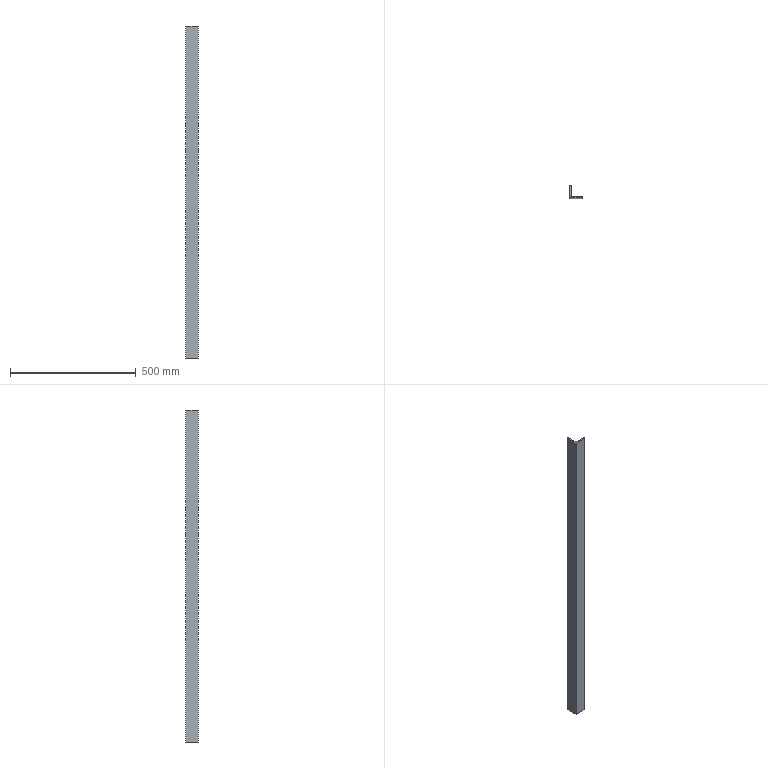Part | SolidWorks | features Extrusion 1 | 1 solid | 11 faces | box 50 x 50 x 1321 mm | volume 751238 mm3 | plane 8 | cylinder 3 | commonest cylinder face diameters 4 x2 11 x1
STEP:
#1=CARTESIAN_POINT('',(4.,50.,-660.4));
#2=VERTEX_POINT('',#1);
#3=CARTESIAN_POINT('',(0.,50.,-660.4));
#4=VERTEX_POINT('',#3);
#5=CARTESIAN_POINT('',(4.,50.,-660.4));
#6=DIRECTION('',(-1.,0.,0.));
#7=VECTOR('',#6,1000.);
#8=LINE('',#5,#7);
#9=EDGE_CURVE('',#2,#4,#8,.T.);
#10=ORIENTED_EDGE('',*,*,#9,.T.);
#11=CARTESIAN_POINT('',(0.,50.,660.4));
#12=VERTEX_POINT('',#11);
#13=CARTESIAN_POINT('',(0.,50.,660.4));
#14=DIRECTION('',(0.,0.,-1.));
#15=VECTOR('',#14,1000.);
#16=LINE('',#13,#15);
#17=EDGE_CURVE('',#12,#4,#16,.T.);
#18=ORIENTED_EDGE('',*,*,#17,.F.);
#19=CARTESIAN_POINT('',(4.,50.,660.4));
#20=VERTEX_POINT('',#19);
#21=CARTESIAN_POINT('',(4.,50.,660.4));
#22=DIRECTION('',(-1.,0.,0.));
#23=VECTOR('',#22,1000.);
#24=LINE('',#21,#23);
#25=EDGE_CURVE('',#20,#12,#24,.T.);
#26=ORIENTED_EDGE('',*,*,#25,.F.);
#27=CARTESIAN_POINT('',(4.,50.,660.4));
#28=DIRECTION('',(0.,0.,-1.));
#29=VECTOR('',#28,1000.);
#30=LINE('',#27,#29);
#31=EDGE_CURVE('',#20,#2,#30,.T.);
#32=ORIENTED_EDGE('',*,*,#31,.T.);
#33=EDGE_LOOP('',(#10,#18,#26,#32));
#34=FACE_OUTER_BOUND('',#33,.T.);
#35=CARTESIAN_POINT('',(4.,50.,660.4));
#36=DIRECTION('',(0.,-1.,0.));
#37=DIRECTION('',(0.,0.,-1.));
#38=AXIS2_PLACEMENT_3D('',#35,#36,#37);
#39=PLANE('',#38);
#40=ADVANCED_FACE('',(#34),#39,.F.);
#41=CARTESIAN_POINT('',(0.,0.,-660.4));
#42=VERTEX_POINT('',#41);
#43=CARTESIAN_POINT('',(0.,50.,-660.4));
#44=DIRECTION('',(0.,-1.,0.));
#45=VECTOR('',#44,1000.);
#46=LINE('',#43,#45);
#47=EDGE_CURVE('',#4,#42,#46,.T.);
#48=ORIENTED_EDGE('',*,*,#47,.T.);
#49=CARTESIAN_POINT('',(0.,0.,660.4));
#50=VERTEX_POINT('',#49);
#51=CARTESIAN_POINT('',(0.,0.,660.4));
#52=DIRECTION('',(0.,0.,-1.));
#53=VECTOR('',#52,1000.);
#54=LINE('',#51,#53);
#55=EDGE_CURVE('',#50,#42,#54,.T.);
#56=ORIENTED_EDGE('',*,*,#55,.F.);
#57=CARTESIAN_POINT('',(0.,50.,660.4));
#58=DIRECTION('',(0.,-1.,0.));
#59=VECTOR('',#58,1000.);
#60=LINE('',#57,#59);
#61=EDGE_CURVE('',#12,#50,#60,.T.);
#62=ORIENTED_EDGE('',*,*,#61,.F.);
#63=ORIENTED_EDGE('',*,*,#17,.T.);
#64=EDGE_LOOP('',(#48,#56,#62,#63));
#65=FACE_OUTER_BOUND('',#64,.T.);
#66=CARTESIAN_POINT('',(0.,50.,660.4));
#67=DIRECTION('',(1.,0.,0.));
#68=DIRECTION('',(0.,1.,0.));
#69=AXIS2_PLACEMENT_3D('',#66,#67,#68);
#70=PLANE('',#69);
#71=ADVANCED_FACE('',(#65),#70,.F.);
#72=CARTESIAN_POINT('',(50.,0.,-660.4));
#73=VERTEX_POINT('',#72);
#74=CARTESIAN_POINT('',(0.,0.,-660.4));
#75=DIRECTION('',(1.,0.,0.));
#76=VECTOR('',#75,1000.);
#77=LINE('',#74,#76);
#78=EDGE_CURVE('',#42,#73,#77,.T.);
#79=ORIENTED_EDGE('',*,*,#78,.T.);
#80=CARTESIAN_POINT('',(50.,0.,660.4));
#81=VERTEX_POINT('',#80);
#82=CARTESIAN_POINT('',(50.,0.,660.4));
#83=DIRECTION('',(0.,0.,-1.));
#84=VECTOR('',#83,1000.);
#85=LINE('',#82,#84);
#86=EDGE_CURVE('',#81,#73,#85,.T.);
#87=ORIENTED_EDGE('',*,*,#86,.F.);
#88=CARTESIAN_POINT('',(0.,0.,660.4));
#89=DIRECTION('',(1.,0.,0.));
#90=VECTOR('',#89,1000.);
#91=LINE('',#88,#90);
#92=EDGE_CURVE('',#50,#81,#91,.T.);
#93=ORIENTED_EDGE('',*,*,#92,.F.);
#94=ORIENTED_EDGE('',*,*,#55,.T.);
#95=EDGE_LOOP('',(#79,#87,#93,#94));
#96=FACE_OUTER_BOUND('',#95,.T.);
#97=CARTESIAN_POINT('',(0.,0.,660.4));
#98=DIRECTION('',(0.,1.,0.));
#99=DIRECTION('',(0.,0.,1.));
#100=AXIS2_PLACEMENT_3D('',#97,#98,#99);
#101=PLANE('',#100);
#102=ADVANCED_FACE('',(#96),#101,.F.);
#103=CARTESIAN_POINT('',(50.,4.,-660.4));
#104=VERTEX_POINT('',#103);
#105=CARTESIAN_POINT('',(50.,0.,-660.4));
#106=DIRECTION('',(0.,1.,0.));
#107=VECTOR('',#106,1000.);
#108=LINE('',#105,#107);
#109=EDGE_CURVE('',#73,#104,#108,.T.);
#110=ORIENTED_EDGE('',*,*,#109,.T.);
#111=CARTESIAN_POINT('',(50.,4.,660.4));
#112=VERTEX_POINT('',#111);
#113=CARTESIAN_POINT('',(50.,4.,660.4));
#114=DIRECTION('',(0.,0.,-1.));
#115=VECTOR('',#114,1000.);
#116=LINE('',#113,#115);
#117=EDGE_CURVE('',#112,#104,#116,.T.);
#118=ORIENTED_EDGE('',*,*,#117,.F.);
#119=CARTESIAN_POINT('',(50.,0.,660.4));
#120=DIRECTION('',(0.,1.,0.));
#121=VECTOR('',#120,1000.);
#122=LINE('',#119,#121);
#123=EDGE_CURVE('',#81,#112,#122,.T.);
#124=ORIENTED_EDGE('',*,*,#123,.F.);
#125=ORIENTED_EDGE('',*,*,#86,.T.);
#126=EDGE_LOOP('',(#110,#118,#124,#125));
#127=FACE_OUTER_BOUND('',#126,.T.);
#128=CARTESIAN_POINT('',(50.,0.,660.4));
#129=DIRECTION('',(-1.,0.,0.));
#130=DIRECTION('',(0.,0.,1.));
#131=AXIS2_PLACEMENT_3D('',#128,#129,#130);
#132=PLANE('',#131);
#133=ADVANCED_FACE('',(#127),#132,.F.);
#134=CARTESIAN_POINT('',(48.,6.,-660.4));
#135=VERTEX_POINT('',#134);
#136=CARTESIAN_POINT('',(48.,4.,-660.4));
#137=DIRECTION('',(0.,0.,1.));
#138=DIRECTION('',(1.,0.,0.));
#139=AXIS2_PLACEMENT_3D('',#136,#137,#138);
#140=CIRCLE('',#139,2.);
#141=EDGE_CURVE('',#104,#135,#140,.T.);
#142=ORIENTED_EDGE('',*,*,#141,.T.);
#143=CARTESIAN_POINT('',(48.,6.,660.4));
#144=VERTEX_POINT('',#143);
#145=CARTESIAN_POINT('',(48.,6.,660.4));
#146=DIRECTION('',(0.,0.,-1.));
#147=VECTOR('',#146,1000.);
#148=LINE('',#145,#147);
#149=EDGE_CURVE('',#144,#135,#148,.T.);
#150=ORIENTED_EDGE('',*,*,#149,.F.);
#151=CARTESIAN_POINT('',(48.,4.,660.4));
#152=DIRECTION('',(0.,0.,1.));
#153=DIRECTION('',(1.,0.,0.));
#154=AXIS2_PLACEMENT_3D('',#151,#152,#153);
#155=CIRCLE('',#154,2.);
#156=EDGE_CURVE('',#112,#144,#155,.T.);
#157=ORIENTED_EDGE('',*,*,#156,.F.);
#158=ORIENTED_EDGE('',*,*,#117,.T.);
#159=EDGE_LOOP('',(#142,#150,#157,#158));
#160=FACE_OUTER_BOUND('',#159,.T.);
#161=CARTESIAN_POINT('',(48.,4.,660.4));
#162=DIRECTION('',(0.,0.,-1.));
#163=DIRECTION('',(-1.,0.,0.));
#164=AXIS2_PLACEMENT_3D('',#161,#162,#163);
#165=CYLINDRICAL_SURFACE('',#164,2.);
#166=ADVANCED_FACE('',(#160),#165,.T.);
#167=CARTESIAN_POINT('',(11.5,6.,-660.4));
#168=VERTEX_POINT('',#167);
#169=CARTESIAN_POINT('',(48.,6.,-660.4));
#170=DIRECTION('',(-1.,0.,0.));
#171=VECTOR('',#170,1000.);
#172=LINE('',#169,#171);
#173=EDGE_CURVE('',#135,#168,#172,.T.);
#174=ORIENTED_EDGE('',*,*,#173,.T.);
#175=CARTESIAN_POINT('',(11.5,6.,660.4));
#176=VERTEX_POINT('',#175);
#177=CARTESIAN_POINT('',(11.5,6.,660.4));
#178=DIRECTION('',(0.,0.,-1.));
#179=VECTOR('',#178,1000.);
#180=LINE('',#177,#179);
#181=EDGE_CURVE('',#176,#168,#180,.T.);
#182=ORIENTED_EDGE('',*,*,#181,.F.);
#183=CARTESIAN_POINT('',(48.,6.,660.4));
#184=DIRECTION('',(-1.,0.,0.));
#185=VECTOR('',#184,1000.);
#186=LINE('',#183,#185);
#187=EDGE_CURVE('',#144,#176,#186,.T.);
#188=ORIENTED_EDGE('',*,*,#187,.F.);
#189=ORIENTED_EDGE('',*,*,#149,.T.);
#190=EDGE_LOOP('',(#174,#182,#188,#189));
#191=FACE_OUTER_BOUND('',#190,.T.);
#192=CARTESIAN_POINT('',(48.,6.,660.4));
#193=DIRECTION('',(0.,-1.,0.));
#194=DIRECTION('',(1.,0.,0.));
#195=AXIS2_PLACEMENT_3D('',#192,#193,#194);
#196=PLANE('',#195);
#197=ADVANCED_FACE('',(#191),#196,.F.);
#198=CARTESIAN_POINT('',(6.,11.5,-660.4));
#199=VERTEX_POINT('',#198);
#200=CARTESIAN_POINT('',(11.5,11.5,-660.4));
#201=DIRECTION('',(0.,0.,-1.));
#202=DIRECTION('',(-1.,0.,0.));
#203=AXIS2_PLACEMENT_3D('',#200,#201,#202);
#204=CIRCLE('',#203,5.5);
#205=EDGE_CURVE('',#168,#199,#204,.T.);
#206=ORIENTED_EDGE('',*,*,#205,.T.);
#207=CARTESIAN_POINT('',(6.,11.5,660.4));
#208=VERTEX_POINT('',#207);
#209=CARTESIAN_POINT('',(6.,11.5,660.4));
#210=DIRECTION('',(0.,0.,-1.));
#211=VECTOR('',#210,1000.);
#212=LINE('',#209,#211);
#213=EDGE_CURVE('',#208,#199,#212,.T.);
#214=ORIENTED_EDGE('',*,*,#213,.F.);
#215=CARTESIAN_POINT('',(11.5,11.5,660.4));
#216=DIRECTION('',(0.,0.,-1.));
#217=DIRECTION('',(-1.,0.,0.));
#218=AXIS2_PLACEMENT_3D('',#215,#216,#217);
#219=CIRCLE('',#218,5.5);
#220=EDGE_CURVE('',#176,#208,#219,.T.);
#221=ORIENTED_EDGE('',*,*,#220,.F.);
#222=ORIENTED_EDGE('',*,*,#181,.T.);
#223=EDGE_LOOP('',(#206,#214,#221,#222));
#224=FACE_OUTER_BOUND('',#223,.T.);
#225=CARTESIAN_POINT('',(11.5,11.5,660.4));
#226=DIRECTION('',(0.,0.,-1.));
#227=DIRECTION('',(-1.,0.,0.));
#228=AXIS2_PLACEMENT_3D('',#225,#226,#227);
#229=CYLINDRICAL_SURFACE('',#228,5.5);
#230=ADVANCED_FACE('',(#224),#229,.F.);
#231=CARTESIAN_POINT('',(6.,48.,-660.4));
#232=VERTEX_POINT('',#231);
#233=CARTESIAN_POINT('',(6.,11.5,-660.4));
#234=DIRECTION('',(0.,1.,0.));
#235=VECTOR('',#234,1000.);
#236=LINE('',#233,#235);
#237=EDGE_CURVE('',#199,#232,#236,.T.);
#238=ORIENTED_EDGE('',*,*,#237,.T.);
#239=CARTESIAN_POINT('',(6.,48.,660.4));
#240=VERTEX_POINT('',#239);
#241=CARTESIAN_POINT('',(6.,48.,660.4));
#242=DIRECTION('',(0.,0.,-1.));
#243=VECTOR('',#242,1000.);
#244=LINE('',#241,#243);
#245=EDGE_CURVE('',#240,#232,#244,.T.);
#246=ORIENTED_EDGE('',*,*,#245,.F.);
#247=CARTESIAN_POINT('',(6.,11.5,660.4));
#248=DIRECTION('',(0.,1.,0.));
#249=VECTOR('',#248,1000.);
#250=LINE('',#247,#249);
#251=EDGE_CURVE('',#208,#240,#250,.T.);
#252=ORIENTED_EDGE('',*,*,#251,.F.);
#253=ORIENTED_EDGE('',*,*,#213,.T.);
#254=EDGE_LOOP('',(#238,#246,#252,#253));
#255=FACE_OUTER_BOUND('',#254,.T.);
#256=CARTESIAN_POINT('',(6.,11.5,660.4));
#257=DIRECTION('',(-1.,0.,0.));
#258=DIRECTION('',(0.,-1.,0.));
#259=AXIS2_PLACEMENT_3D('',#256,#257,#258);
#260=PLANE('',#259);
#261=ADVANCED_FACE('',(#255),#260,.F.);
#262=CARTESIAN_POINT('',(4.,48.,-660.4));
#263=DIRECTION('',(0.,0.,1.));
#264=DIRECTION('',(1.,0.,0.));
#265=AXIS2_PLACEMENT_3D('',#262,#263,#264);
#266=CIRCLE('',#265,2.);
#267=EDGE_CURVE('',#232,#2,#266,.T.);
#268=ORIENTED_EDGE('',*,*,#267,.T.);
#269=ORIENTED_EDGE('',*,*,#31,.F.);
#270=CARTESIAN_POINT('',(4.,48.,660.4));
#271=DIRECTION('',(0.,0.,1.));
#272=DIRECTION('',(1.,0.,0.));
#273=AXIS2_PLACEMENT_3D('',#270,#271,#272);
#274=CIRCLE('',#273,2.);
#275=EDGE_CURVE('',#240,#20,#274,.T.);
#276=ORIENTED_EDGE('',*,*,#275,.F.);
#277=ORIENTED_EDGE('',*,*,#245,.T.);
#278=EDGE_LOOP('',(#268,#269,#276,#277));
#279=FACE_OUTER_BOUND('',#278,.T.);
#280=CARTESIAN_POINT('',(4.,48.,660.4));
#281=DIRECTION('',(0.,0.,-1.));
#282=DIRECTION('',(-1.,0.,0.));
#283=AXIS2_PLACEMENT_3D('',#280,#281,#282);
#284=CYLINDRICAL_SURFACE('',#283,2.);
#285=ADVANCED_FACE('',(#279),#284,.T.);
#286=ORIENTED_EDGE('',*,*,#25,.T.);
#287=ORIENTED_EDGE('',*,*,#61,.T.);
#288=ORIENTED_EDGE('',*,*,#92,.T.);
#289=ORIENTED_EDGE('',*,*,#123,.T.);
#290=ORIENTED_EDGE('',*,*,#156,.T.);
#291=ORIENTED_EDGE('',*,*,#187,.T.);
#292=ORIENTED_EDGE('',*,*,#220,.T.);
#293=ORIENTED_EDGE('',*,*,#251,.T.);
#294=ORIENTED_EDGE('',*,*,#275,.T.);
#295=EDGE_LOOP('',(#286,#287,#288,#289,#290,#291,#292,#293,#294));
#296=FACE_OUTER_BOUND('',#295,.T.);
#297=CARTESIAN_POINT('',(48.,4.,660.4));
#298=DIRECTION('',(0.,0.,1.));
#299=DIRECTION('',(1.,0.,0.));
#300=AXIS2_PLACEMENT_3D('',#297,#298,#299);
#301=PLANE('',#300);
#302=ADVANCED_FACE('',(#296),#301,.T.);
#303=ORIENTED_EDGE('',*,*,#9,.F.);
#304=ORIENTED_EDGE('',*,*,#267,.F.);
#305=ORIENTED_EDGE('',*,*,#237,.F.);
#306=ORIENTED_EDGE('',*,*,#205,.F.);
#307=ORIENTED_EDGE('',*,*,#173,.F.);
#308=ORIENTED_EDGE('',*,*,#141,.F.);
#309=ORIENTED_EDGE('',*,*,#109,.F.);
#310=ORIENTED_EDGE('',*,*,#78,.F.);
#311=ORIENTED_EDGE('',*,*,#47,.F.);
#312=EDGE_LOOP('',(#303,#304,#305,#306,#307,#308,#309,#310,#311));
#313=FACE_OUTER_BOUND('',#312,.T.);
#314=CARTESIAN_POINT('',(48.,4.,-660.4));
#315=DIRECTION('',(0.,0.,1.));
#316=DIRECTION('',(1.,0.,0.));
#317=AXIS2_PLACEMENT_3D('',#314,#315,#316);
#318=PLANE('',#317);
#319=ADVANCED_FACE('',(#313),#318,.F.);
#320=CLOSED_SHELL('',(#40,#71,#102,#133,#166,#197,#230,#261,#285,#302,#319));
#321=MANIFOLD_SOLID_BREP('',#320);
#322=CARTESIAN_POINT('',(0.,0.,0.));
#323=DIRECTION('',(0.,0.,1.));
#324=DIRECTION('',(1.,0.,0.));
#325=AXIS2_PLACEMENT_3D('',#322,#323,#324);
#326=(LENGTH_UNIT()NAMED_UNIT(*)SI_UNIT(.MILLI.,.METRE.));
#327=UNCERTAINTY_MEASURE_WITH_UNIT(LENGTH_MEASURE(0.00001),#326,'','');
#328=(NAMED_UNIT(*)PLANE_ANGLE_UNIT()SI_UNIT($,.RADIAN.));
#329=(NAMED_UNIT(*)SI_UNIT($,.STERADIAN.)SOLID_ANGLE_UNIT());
#330=(GEOMETRIC_REPRESENTATION_CONTEXT(3)GLOBAL_UNCERTAINTY_ASSIGNED_CONTEXT((#327))GLOBAL_UNIT_ASSIGNED_CONTEXT((#326,#328,#329))REPRESENTATION_CONTEXT('',''));
#331=ADVANCED_BREP_SHAPE_REPRESENTATION('',(#321,#325),#330);